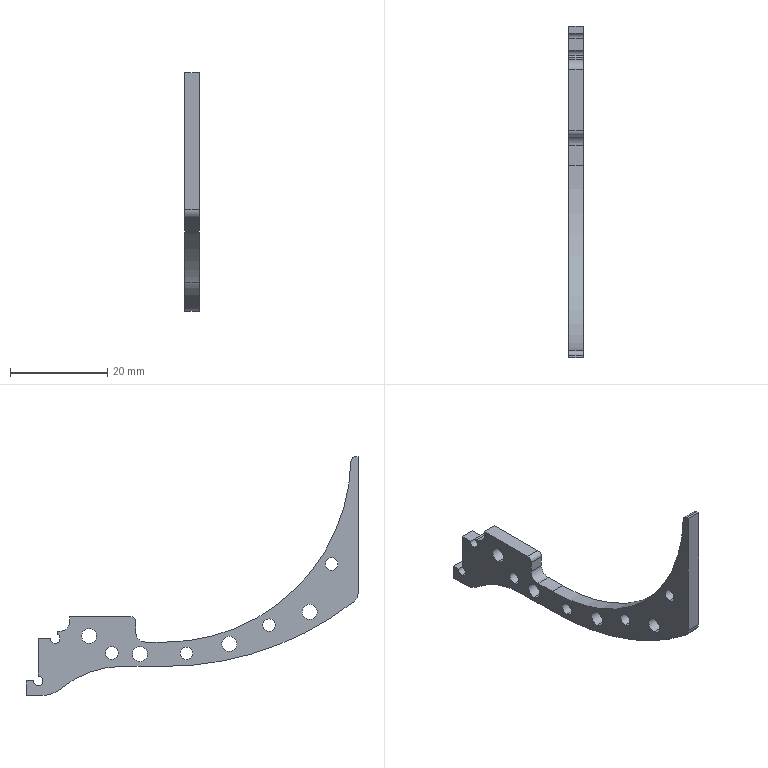Part | SolidWorks | features Fillet 2, Extrusion 1, ICE 1 | 1 solid | 45 faces | box 3 x 68.45 x 49.25 mm | volume 1803 mm3 | cylinder 29 | plane 16 | commonest cylinder face diameters 2.6 x8 3.1 x8 2 x6 4 x3 11.1 x1 40 x1
STEP:
#1=CARTESIAN_POINT('',(0.,27.25,-22.25));
#2=VERTEX_POINT('',#1);
#3=CARTESIAN_POINT('',(0.,26.25,-23.25));
#4=VERTEX_POINT('',#3);
#5=CARTESIAN_POINT('',(0.,26.25,-22.25));
#6=DIRECTION('',(-1.,0.,0.));
#7=DIRECTION('',(0.,0.,-1.));
#8=AXIS2_PLACEMENT_3D('',#5,#6,#7);
#9=CIRCLE('',#8,1.);
#10=EDGE_CURVE('',#2,#4,#9,.T.);
#11=ORIENTED_EDGE('',*,*,#10,.T.);
#12=CARTESIAN_POINT('',(3.,26.25,-23.25));
#13=VERTEX_POINT('',#12);
#14=CARTESIAN_POINT('',(0.,26.25,-23.25));
#15=DIRECTION('',(1.,0.,0.));
#16=VECTOR('',#15,1000.);
#17=LINE('',#14,#16);
#18=EDGE_CURVE('',#4,#13,#17,.T.);
#19=ORIENTED_EDGE('',*,*,#18,.T.);
#20=CARTESIAN_POINT('',(3.,27.25,-22.25));
#21=VERTEX_POINT('',#20);
#22=CARTESIAN_POINT('',(3.,26.25,-22.25));
#23=DIRECTION('',(-1.,0.,0.));
#24=DIRECTION('',(0.,0.,-1.));
#25=AXIS2_PLACEMENT_3D('',#22,#23,#24);
#26=CIRCLE('',#25,1.);
#27=EDGE_CURVE('',#21,#13,#26,.T.);
#28=ORIENTED_EDGE('',*,*,#27,.F.);
#29=CARTESIAN_POINT('',(0.,27.25,-22.25));
#30=DIRECTION('',(1.,0.,0.));
#31=VECTOR('',#30,1000.);
#32=LINE('',#29,#31);
#33=EDGE_CURVE('',#2,#21,#32,.T.);
#34=ORIENTED_EDGE('',*,*,#33,.F.);
#35=EDGE_LOOP('',(#11,#19,#28,#34));
#36=FACE_OUTER_BOUND('',#35,.T.);
#37=CARTESIAN_POINT('',(0.,26.25,-22.25));
#38=DIRECTION('',(1.,0.,0.));
#39=DIRECTION('',(0.,0.,-1.));
#40=AXIS2_PLACEMENT_3D('',#37,#38,#39);
#41=CYLINDRICAL_SURFACE('',#40,1.);
#42=ADVANCED_FACE('',(#36),#41,.F.);
#43=CARTESIAN_POINT('',(0.,23.75,-13.5));
#44=VERTEX_POINT('',#43);
#45=CARTESIAN_POINT('',(0.,22.75,-14.5));
#46=VERTEX_POINT('',#45);
#47=CARTESIAN_POINT('',(0.,22.75,-13.5));
#48=DIRECTION('',(-1.,0.,0.));
#49=DIRECTION('',(0.,0.,-1.));
#50=AXIS2_PLACEMENT_3D('',#47,#48,#49);
#51=CIRCLE('',#50,1.);
#52=EDGE_CURVE('',#44,#46,#51,.T.);
#53=ORIENTED_EDGE('',*,*,#52,.T.);
#54=CARTESIAN_POINT('',(3.,22.75,-14.5));
#55=VERTEX_POINT('',#54);
#56=CARTESIAN_POINT('',(0.,22.75,-14.5));
#57=DIRECTION('',(1.,0.,0.));
#58=VECTOR('',#57,1000.);
#59=LINE('',#56,#58);
#60=EDGE_CURVE('',#46,#55,#59,.T.);
#61=ORIENTED_EDGE('',*,*,#60,.T.);
#62=CARTESIAN_POINT('',(3.,23.75,-13.5));
#63=VERTEX_POINT('',#62);
#64=CARTESIAN_POINT('',(3.,22.75,-13.5));
#65=DIRECTION('',(-1.,0.,0.));
#66=DIRECTION('',(0.,0.,-1.));
#67=AXIS2_PLACEMENT_3D('',#64,#65,#66);
#68=CIRCLE('',#67,1.);
#69=EDGE_CURVE('',#63,#55,#68,.T.);
#70=ORIENTED_EDGE('',*,*,#69,.F.);
#71=CARTESIAN_POINT('',(0.,23.75,-13.5));
#72=DIRECTION('',(1.,0.,0.));
#73=VECTOR('',#72,1000.);
#74=LINE('',#71,#73);
#75=EDGE_CURVE('',#44,#63,#74,.T.);
#76=ORIENTED_EDGE('',*,*,#75,.F.);
#77=EDGE_LOOP('',(#53,#61,#70,#76));
#78=FACE_OUTER_BOUND('',#77,.T.);
#79=CARTESIAN_POINT('',(0.,22.75,-13.5));
#80=DIRECTION('',(1.,0.,0.));
#81=DIRECTION('',(0.,0.,-1.));
#82=AXIS2_PLACEMENT_3D('',#79,#80,#81);
#83=CYLINDRICAL_SURFACE('',#82,1.);
#84=ADVANCED_FACE('',(#78),#83,.F.);
#85=CARTESIAN_POINT('',(3.,15.75,-14.55));
#86=VERTEX_POINT('',#85);
#87=CARTESIAN_POINT('',(3.,15.75,-11.45));
#88=VERTEX_POINT('',#87);
#89=CARTESIAN_POINT('',(3.,15.75,-13.));
#90=DIRECTION('',(-1.,0.,0.));
#91=DIRECTION('',(0.,0.,-1.));
#92=AXIS2_PLACEMENT_3D('',#89,#90,#91);
#93=CIRCLE('',#92,1.55);
#94=EDGE_CURVE('',#86,#88,#93,.T.);
#95=ORIENTED_EDGE('',*,*,#94,.F.);
#96=CARTESIAN_POINT('',(0.,15.75,-14.55));
#97=VERTEX_POINT('',#96);
#98=CARTESIAN_POINT('',(3.,15.75,-14.55));
#99=DIRECTION('',(-1.,0.,0.));
#100=VECTOR('',#99,1000.);
#101=LINE('',#98,#100);
#102=EDGE_CURVE('',#86,#97,#101,.T.);
#103=ORIENTED_EDGE('',*,*,#102,.T.);
#104=CARTESIAN_POINT('',(0.,15.75,-11.45));
#105=VERTEX_POINT('',#104);
#106=CARTESIAN_POINT('',(0.,15.75,-13.));
#107=DIRECTION('',(-1.,0.,0.));
#108=DIRECTION('',(0.,0.,-1.));
#109=AXIS2_PLACEMENT_3D('',#106,#107,#108);
#110=CIRCLE('',#109,1.55);
#111=EDGE_CURVE('',#97,#105,#110,.T.);
#112=ORIENTED_EDGE('',*,*,#111,.T.);
#113=CARTESIAN_POINT('',(3.,15.75,-11.45));
#114=DIRECTION('',(-1.,0.,0.));
#115=VECTOR('',#114,1000.);
#116=LINE('',#113,#115);
#117=EDGE_CURVE('',#88,#105,#116,.T.);
#118=ORIENTED_EDGE('',*,*,#117,.F.);
#119=EDGE_LOOP('',(#95,#103,#112,#118));
#120=FACE_OUTER_BOUND('',#119,.T.);
#121=CARTESIAN_POINT('',(3.,15.75,-13.));
#122=DIRECTION('',(-1.,0.,0.));
#123=DIRECTION('',(0.,0.,1.));
#124=AXIS2_PLACEMENT_3D('',#121,#122,#123);
#125=CYLINDRICAL_SURFACE('',#124,1.55);
#126=ADVANCED_FACE('',(#120),#125,.F.);
#127=CARTESIAN_POINT('',(3.,-29.75,-6.45));
#128=VERTEX_POINT('',#127);
#129=CARTESIAN_POINT('',(3.,-29.75,-9.55));
#130=VERTEX_POINT('',#129);
#131=CARTESIAN_POINT('',(3.,-29.75,-8.));
#132=DIRECTION('',(1.,0.,0.));
#133=DIRECTION('',(0.,0.,-1.));
#134=AXIS2_PLACEMENT_3D('',#131,#132,#133);
#135=CIRCLE('',#134,1.55);
#136=EDGE_CURVE('',#128,#130,#135,.T.);
#137=ORIENTED_EDGE('',*,*,#136,.T.);
#138=CARTESIAN_POINT('',(0.,-29.75,-9.55));
#139=VERTEX_POINT('',#138);
#140=CARTESIAN_POINT('',(3.,-29.75,-9.55));
#141=DIRECTION('',(-1.,0.,0.));
#142=VECTOR('',#141,1000.);
#143=LINE('',#140,#142);
#144=EDGE_CURVE('',#130,#139,#143,.T.);
#145=ORIENTED_EDGE('',*,*,#144,.T.);
#146=CARTESIAN_POINT('',(0.,-29.75,-6.45));
#147=VERTEX_POINT('',#146);
#148=CARTESIAN_POINT('',(0.,-29.75,-8.));
#149=DIRECTION('',(1.,0.,0.));
#150=DIRECTION('',(0.,0.,-1.));
#151=AXIS2_PLACEMENT_3D('',#148,#149,#150);
#152=CIRCLE('',#151,1.55);
#153=EDGE_CURVE('',#147,#139,#152,.T.);
#154=ORIENTED_EDGE('',*,*,#153,.F.);
#155=CARTESIAN_POINT('',(3.,-29.75,-6.45));
#156=DIRECTION('',(-1.,0.,0.));
#157=VECTOR('',#156,1000.);
#158=LINE('',#155,#157);
#159=EDGE_CURVE('',#128,#147,#158,.T.);
#160=ORIENTED_EDGE('',*,*,#159,.F.);
#161=EDGE_LOOP('',(#137,#145,#154,#160));
#162=FACE_OUTER_BOUND('',#161,.T.);
#163=CARTESIAN_POINT('',(3.,-29.75,-8.));
#164=DIRECTION('',(-1.,0.,0.));
#165=DIRECTION('',(0.,0.,1.));
#166=AXIS2_PLACEMENT_3D('',#163,#164,#165);
#167=CYLINDRICAL_SURFACE('',#166,1.55);
#168=ADVANCED_FACE('',(#162),#167,.F.);
#169=CARTESIAN_POINT('',(3.,-4.324,-15.27));
#170=VERTEX_POINT('',#169);
#171=CARTESIAN_POINT('',(3.,-4.324,-17.87));
#172=VERTEX_POINT('',#171);
#173=CARTESIAN_POINT('',(3.,-4.324,-16.57));
#174=DIRECTION('',(1.,0.,0.));
#175=DIRECTION('',(0.,0.,-1.));
#176=AXIS2_PLACEMENT_3D('',#173,#174,#175);
#177=CIRCLE('',#176,1.3);
#178=EDGE_CURVE('',#170,#172,#177,.T.);
#179=ORIENTED_EDGE('',*,*,#178,.T.);
#180=CARTESIAN_POINT('',(0.,-4.324,-17.87));
#181=VERTEX_POINT('',#180);
#182=CARTESIAN_POINT('',(3.,-4.324,-17.87));
#183=DIRECTION('',(-1.,0.,0.));
#184=VECTOR('',#183,1000.);
#185=LINE('',#182,#184);
#186=EDGE_CURVE('',#172,#181,#185,.T.);
#187=ORIENTED_EDGE('',*,*,#186,.T.);
#188=CARTESIAN_POINT('',(0.,-4.324,-15.27));
#189=VERTEX_POINT('',#188);
#190=CARTESIAN_POINT('',(0.,-4.324,-16.57));
#191=DIRECTION('',(1.,0.,0.));
#192=DIRECTION('',(0.,0.,-1.));
#193=AXIS2_PLACEMENT_3D('',#190,#191,#192);
#194=CIRCLE('',#193,1.3);
#195=EDGE_CURVE('',#189,#181,#194,.T.);
#196=ORIENTED_EDGE('',*,*,#195,.F.);
#197=CARTESIAN_POINT('',(3.,-4.324,-15.27));
#198=DIRECTION('',(-1.,0.,0.));
#199=VECTOR('',#198,1000.);
#200=LINE('',#197,#199);
#201=EDGE_CURVE('',#170,#189,#200,.T.);
#202=ORIENTED_EDGE('',*,*,#201,.F.);
#203=EDGE_LOOP('',(#179,#187,#196,#202));
#204=FACE_OUTER_BOUND('',#203,.T.);
#205=CARTESIAN_POINT('',(3.,-4.324,-16.57));
#206=DIRECTION('',(-1.,0.,0.));
#207=DIRECTION('',(0.,0.,1.));
#208=AXIS2_PLACEMENT_3D('',#205,#206,#207);
#209=CYLINDRICAL_SURFACE('',#208,1.3);
#210=ADVANCED_FACE('',(#204),#209,.F.);
#211=CARTESIAN_POINT('',(3.,-13.171,-13.066));
#212=VERTEX_POINT('',#211);
#213=CARTESIAN_POINT('',(3.,-13.171,-16.166));
#214=VERTEX_POINT('',#213);
#215=CARTESIAN_POINT('',(3.,-13.171,-14.616));
#216=DIRECTION('',(1.,0.,0.));
#217=DIRECTION('',(0.,0.,-1.));
#218=AXIS2_PLACEMENT_3D('',#215,#216,#217);
#219=CIRCLE('',#218,1.55);
#220=EDGE_CURVE('',#212,#214,#219,.T.);
#221=ORIENTED_EDGE('',*,*,#220,.T.);
#222=CARTESIAN_POINT('',(0.,-13.171,-16.166));
#223=VERTEX_POINT('',#222);
#224=CARTESIAN_POINT('',(3.,-13.171,-16.166));
#225=DIRECTION('',(-1.,0.,0.));
#226=VECTOR('',#225,1000.);
#227=LINE('',#224,#226);
#228=EDGE_CURVE('',#214,#223,#227,.T.);
#229=ORIENTED_EDGE('',*,*,#228,.T.);
#230=CARTESIAN_POINT('',(0.,-13.171,-13.066));
#231=VERTEX_POINT('',#230);
#232=CARTESIAN_POINT('',(0.,-13.171,-14.616));
#233=DIRECTION('',(1.,0.,0.));
#234=DIRECTION('',(0.,0.,-1.));
#235=AXIS2_PLACEMENT_3D('',#232,#233,#234);
#236=CIRCLE('',#235,1.55);
#237=EDGE_CURVE('',#231,#223,#236,.T.);
#238=ORIENTED_EDGE('',*,*,#237,.F.);
#239=CARTESIAN_POINT('',(3.,-13.171,-13.066));
#240=DIRECTION('',(-1.,0.,0.));
#241=VECTOR('',#240,1000.);
#242=LINE('',#239,#241);
#243=EDGE_CURVE('',#212,#231,#242,.T.);
#244=ORIENTED_EDGE('',*,*,#243,.F.);
#245=EDGE_LOOP('',(#221,#229,#238,#244));
#246=FACE_OUTER_BOUND('',#245,.T.);
#247=CARTESIAN_POINT('',(3.,-13.171,-14.616));
#248=DIRECTION('',(-1.,0.,0.));
#249=DIRECTION('',(0.,0.,1.));
#250=AXIS2_PLACEMENT_3D('',#247,#248,#249);
#251=CYLINDRICAL_SURFACE('',#250,1.55);
#252=ADVANCED_FACE('',(#246),#251,.F.);
#253=CARTESIAN_POINT('',(3.,-21.368,-9.457));
#254=VERTEX_POINT('',#253);
#255=CARTESIAN_POINT('',(3.,-21.368,-12.057));
#256=VERTEX_POINT('',#255);
#257=CARTESIAN_POINT('',(3.,-21.368,-10.757));
#258=DIRECTION('',(1.,0.,0.));
#259=DIRECTION('',(0.,0.,-1.));
#260=AXIS2_PLACEMENT_3D('',#257,#258,#259);
#261=CIRCLE('',#260,1.3);
#262=EDGE_CURVE('',#254,#256,#261,.T.);
#263=ORIENTED_EDGE('',*,*,#262,.T.);
#264=CARTESIAN_POINT('',(0.,-21.368,-12.057));
#265=VERTEX_POINT('',#264);
#266=CARTESIAN_POINT('',(3.,-21.368,-12.057));
#267=DIRECTION('',(-1.,0.,0.));
#268=VECTOR('',#267,1000.);
#269=LINE('',#266,#268);
#270=EDGE_CURVE('',#256,#265,#269,.T.);
#271=ORIENTED_EDGE('',*,*,#270,.T.);
#272=CARTESIAN_POINT('',(0.,-21.368,-9.457));
#273=VERTEX_POINT('',#272);
#274=CARTESIAN_POINT('',(0.,-21.368,-10.757));
#275=DIRECTION('',(1.,0.,0.));
#276=DIRECTION('',(0.,0.,-1.));
#277=AXIS2_PLACEMENT_3D('',#274,#275,#276);
#278=CIRCLE('',#277,1.3);
#279=EDGE_CURVE('',#273,#265,#278,.T.);
#280=ORIENTED_EDGE('',*,*,#279,.F.);
#281=CARTESIAN_POINT('',(3.,-21.368,-9.457));
#282=DIRECTION('',(-1.,0.,0.));
#283=VECTOR('',#282,1000.);
#284=LINE('',#281,#283);
#285=EDGE_CURVE('',#254,#273,#284,.T.);
#286=ORIENTED_EDGE('',*,*,#285,.F.);
#287=EDGE_LOOP('',(#263,#271,#280,#286));
#288=FACE_OUTER_BOUND('',#287,.T.);
#289=CARTESIAN_POINT('',(3.,-21.368,-10.757));
#290=DIRECTION('',(-1.,0.,0.));
#291=DIRECTION('',(0.,0.,1.));
#292=AXIS2_PLACEMENT_3D('',#289,#290,#291);
#293=CYLINDRICAL_SURFACE('',#292,1.3);
#294=ADVANCED_FACE('',(#288),#293,.F.);
#295=CARTESIAN_POINT('',(3.,-34.25,3.128));
#296=VERTEX_POINT('',#295);
#297=CARTESIAN_POINT('',(3.,-34.25,0.5285));
#298=VERTEX_POINT('',#297);
#299=CARTESIAN_POINT('',(3.,-34.25,1.828));
#300=DIRECTION('',(1.,0.,0.));
#301=DIRECTION('',(0.,0.,-1.));
#302=AXIS2_PLACEMENT_3D('',#299,#300,#301);
#303=CIRCLE('',#302,1.3);
#304=EDGE_CURVE('',#296,#298,#303,.T.);
#305=ORIENTED_EDGE('',*,*,#304,.T.);
#306=CARTESIAN_POINT('',(0.,-34.25,0.5285));
#307=VERTEX_POINT('',#306);
#308=CARTESIAN_POINT('',(3.,-34.25,0.5285));
#309=DIRECTION('',(-1.,0.,0.));
#310=VECTOR('',#309,1000.);
#311=LINE('',#308,#310);
#312=EDGE_CURVE('',#298,#307,#311,.T.);
#313=ORIENTED_EDGE('',*,*,#312,.T.);
#314=CARTESIAN_POINT('',(0.,-34.25,3.128));
#315=VERTEX_POINT('',#314);
#316=CARTESIAN_POINT('',(0.,-34.25,1.828));
#317=DIRECTION('',(1.,0.,0.));
#318=DIRECTION('',(0.,0.,-1.));
#319=AXIS2_PLACEMENT_3D('',#316,#317,#318);
#320=CIRCLE('',#319,1.3);
#321=EDGE_CURVE('',#315,#307,#320,.T.);
#322=ORIENTED_EDGE('',*,*,#321,.F.);
#323=CARTESIAN_POINT('',(3.,-34.25,3.128));
#324=DIRECTION('',(-1.,0.,0.));
#325=VECTOR('',#324,1000.);
#326=LINE('',#323,#325);
#327=EDGE_CURVE('',#296,#315,#326,.T.);
#328=ORIENTED_EDGE('',*,*,#327,.F.);
#329=EDGE_LOOP('',(#305,#313,#322,#328));
#330=FACE_OUTER_BOUND('',#329,.T.);
#331=CARTESIAN_POINT('',(3.,-34.25,1.828));
#332=DIRECTION('',(-1.,0.,0.));
#333=DIRECTION('',(0.,0.,1.));
#334=AXIS2_PLACEMENT_3D('',#331,#332,#333);
#335=CYLINDRICAL_SURFACE('',#334,1.3);
#336=ADVANCED_FACE('',(#330),#335,.F.);
#337=CARTESIAN_POINT('',(3.,5.25,-15.2));
#338=VERTEX_POINT('',#337);
#339=CARTESIAN_POINT('',(3.,5.25,-18.3));
#340=VERTEX_POINT('',#339);
#341=CARTESIAN_POINT('',(3.,5.25,-16.75));
#342=DIRECTION('',(1.,0.,0.));
#343=DIRECTION('',(0.,0.,-1.));
#344=AXIS2_PLACEMENT_3D('',#341,#342,#343);
#345=CIRCLE('',#344,1.55);
#346=EDGE_CURVE('',#338,#340,#345,.T.);
#347=ORIENTED_EDGE('',*,*,#346,.T.);
#348=CARTESIAN_POINT('',(0.,5.25,-18.3));
#349=VERTEX_POINT('',#348);
#350=CARTESIAN_POINT('',(3.,5.25,-18.3));
#351=DIRECTION('',(-1.,0.,0.));
#352=VECTOR('',#351,1000.);
#353=LINE('',#350,#352);
#354=EDGE_CURVE('',#340,#349,#353,.T.);
#355=ORIENTED_EDGE('',*,*,#354,.T.);
#356=CARTESIAN_POINT('',(0.,5.25,-15.2));
#357=VERTEX_POINT('',#356);
#358=CARTESIAN_POINT('',(0.,5.25,-16.75));
#359=DIRECTION('',(1.,0.,0.));
#360=DIRECTION('',(0.,0.,-1.));
#361=AXIS2_PLACEMENT_3D('',#358,#359,#360);
#362=CIRCLE('',#361,1.55);
#363=EDGE_CURVE('',#357,#349,#362,.T.);
#364=ORIENTED_EDGE('',*,*,#363,.F.);
#365=CARTESIAN_POINT('',(3.,5.25,-15.2));
#366=DIRECTION('',(-1.,0.,0.));
#367=VECTOR('',#366,1000.);
#368=LINE('',#365,#367);
#369=EDGE_CURVE('',#338,#357,#368,.T.);
#370=ORIENTED_EDGE('',*,*,#369,.F.);
#371=EDGE_LOOP('',(#347,#355,#364,#370));
#372=FACE_OUTER_BOUND('',#371,.T.);
#373=CARTESIAN_POINT('',(3.,5.25,-16.75));
#374=DIRECTION('',(-1.,0.,0.));
#375=DIRECTION('',(0.,0.,1.));
#376=AXIS2_PLACEMENT_3D('',#373,#374,#375);
#377=CYLINDRICAL_SURFACE('',#376,1.55);
#378=ADVANCED_FACE('',(#372),#377,.F.);
#379=CARTESIAN_POINT('',(3.,11.05,-17.8));
#380=VERTEX_POINT('',#379);
#381=CARTESIAN_POINT('',(3.,11.05,-15.2));
#382=VERTEX_POINT('',#381);
#383=CARTESIAN_POINT('',(3.,11.05,-16.5));
#384=DIRECTION('',(-1.,0.,0.));
#385=DIRECTION('',(0.,0.,-1.));
#386=AXIS2_PLACEMENT_3D('',#383,#384,#385);
#387=CIRCLE('',#386,1.3);
#388=EDGE_CURVE('',#380,#382,#387,.T.);
#389=ORIENTED_EDGE('',*,*,#388,.F.);
#390=CARTESIAN_POINT('',(0.,11.05,-17.8));
#391=VERTEX_POINT('',#390);
#392=CARTESIAN_POINT('',(3.,11.05,-17.8));
#393=DIRECTION('',(-1.,0.,0.));
#394=VECTOR('',#393,1000.);
#395=LINE('',#392,#394);
#396=EDGE_CURVE('',#380,#391,#395,.T.);
#397=ORIENTED_EDGE('',*,*,#396,.T.);
#398=CARTESIAN_POINT('',(0.,11.05,-15.2));
#399=VERTEX_POINT('',#398);
#400=CARTESIAN_POINT('',(0.,11.05,-16.5));
#401=DIRECTION('',(-1.,0.,0.));
#402=DIRECTION('',(0.,0.,-1.));
#403=AXIS2_PLACEMENT_3D('',#400,#401,#402);
#404=CIRCLE('',#403,1.3);
#405=EDGE_CURVE('',#391,#399,#404,.T.);
#406=ORIENTED_EDGE('',*,*,#405,.T.);
#407=CARTESIAN_POINT('',(3.,11.05,-15.2));
#408=DIRECTION('',(-1.,0.,0.));
#409=VECTOR('',#408,1000.);
#410=LINE('',#407,#409);
#411=EDGE_CURVE('',#382,#399,#410,.T.);
#412=ORIENTED_EDGE('',*,*,#411,.F.);
#413=EDGE_LOOP('',(#389,#397,#406,#412));
#414=FACE_OUTER_BOUND('',#413,.T.);
#415=CARTESIAN_POINT('',(3.,11.05,-16.5));
#416=DIRECTION('',(-1.,0.,0.));
#417=DIRECTION('',(0.,0.,1.));
#418=AXIS2_PLACEMENT_3D('',#415,#416,#417);
#419=CYLINDRICAL_SURFACE('',#418,1.3);
#420=ADVANCED_FACE('',(#414),#419,.F.);
#421=CARTESIAN_POINT('',(3.,19.75,-9.));
#422=VERTEX_POINT('',#421);
#423=CARTESIAN_POINT('',(3.,19.75,-10.));
#424=VERTEX_POINT('',#423);
#425=CARTESIAN_POINT('',(3.,19.75,0.));
#426=DIRECTION('',(0.,0.,-1.));
#427=VECTOR('',#426,1000.);
#428=LINE('',#425,#427);
#429=EDGE_CURVE('',#422,#424,#428,.T.);
#430=ORIENTED_EDGE('',*,*,#429,.T.);
#431=CARTESIAN_POINT('',(0.,19.75,-10.));
#432=VERTEX_POINT('',#431);
#433=CARTESIAN_POINT('',(0.,19.75,-10.));
#434=DIRECTION('',(-1.,0.,0.));
#435=VECTOR('',#434,1000.);
#436=LINE('',#433,#435);
#437=EDGE_CURVE('',#424,#432,#436,.T.);
#438=ORIENTED_EDGE('',*,*,#437,.T.);
#439=CARTESIAN_POINT('',(0.,19.75,-9.));
#440=VERTEX_POINT('',#439);
#441=CARTESIAN_POINT('',(0.,19.75,0.));
#442=DIRECTION('',(0.,0.,-1.));
#443=VECTOR('',#442,1000.);
#444=LINE('',#441,#443);
#445=EDGE_CURVE('',#440,#432,#444,.T.);
#446=ORIENTED_EDGE('',*,*,#445,.F.);
#447=CARTESIAN_POINT('',(0.,19.75,-9.));
#448=DIRECTION('',(1.,0.,0.));
#449=VECTOR('',#448,1000.);
#450=LINE('',#447,#449);
#451=EDGE_CURVE('',#440,#422,#450,.T.);
#452=ORIENTED_EDGE('',*,*,#451,.T.);
#453=EDGE_LOOP('',(#430,#438,#446,#452));
#454=FACE_OUTER_BOUND('',#453,.T.);
#455=CARTESIAN_POINT('',(3.,19.75,0.));
#456=DIRECTION('',(0.,1.,0.));
#457=DIRECTION('',(0.,0.,1.));
#458=AXIS2_PLACEMENT_3D('',#455,#456,#457);
#459=PLANE('',#458);
#460=ADVANCED_FACE('',(#454),#459,.T.);
#461=CARTESIAN_POINT('',(3.,6.116,-10.));
#462=VERTEX_POINT('',#461);
#463=CARTESIAN_POINT('',(3.,6.116,-12.25));
#464=VERTEX_POINT('',#463);
#465=CARTESIAN_POINT('',(3.,6.116,0.));
#466=DIRECTION('',(0.,0.,-1.));
#467=VECTOR('',#466,1000.);
#468=LINE('',#465,#467);
#469=EDGE_CURVE('',#462,#464,#468,.T.);
#470=ORIENTED_EDGE('',*,*,#469,.F.);
#471=CARTESIAN_POINT('',(0.,6.116,-10.));
#472=VERTEX_POINT('',#471);
#473=CARTESIAN_POINT('',(0.,6.116,-10.));
#474=DIRECTION('',(-1.,0.,0.));
#475=VECTOR('',#474,1000.);
#476=LINE('',#473,#475);
#477=EDGE_CURVE('',#462,#472,#476,.T.);
#478=ORIENTED_EDGE('',*,*,#477,.T.);
#479=CARTESIAN_POINT('',(0.,6.116,-12.25));
#480=VERTEX_POINT('',#479);
#481=CARTESIAN_POINT('',(0.,6.116,0.));
#482=DIRECTION('',(0.,0.,-1.));
#483=VECTOR('',#482,1000.);
#484=LINE('',#481,#483);
#485=EDGE_CURVE('',#472,#480,#484,.T.);
#486=ORIENTED_EDGE('',*,*,#485,.T.);
#487=CARTESIAN_POINT('',(3.,6.116,-12.25));
#488=DIRECTION('',(1.,0.,0.));
#489=VECTOR('',#488,1000.);
#490=LINE('',#487,#489);
#491=EDGE_CURVE('',#480,#464,#490,.T.);
#492=ORIENTED_EDGE('',*,*,#491,.T.);
#493=EDGE_LOOP('',(#470,#478,#486,#492));
#494=FACE_OUTER_BOUND('',#493,.T.);
#495=CARTESIAN_POINT('',(3.,6.116,0.));
#496=DIRECTION('',(0.,1.,0.));
#497=DIRECTION('',(0.,0.,1.));
#498=AXIS2_PLACEMENT_3D('',#495,#496,#497);
#499=PLANE('',#498);
#500=ADVANCED_FACE('',(#494),#499,.F.);
#501=CARTESIAN_POINT('',(3.,0.,-14.25));
#502=VERTEX_POINT('',#501);
#503=CARTESIAN_POINT('',(3.,4.116,-14.25));
#504=VERTEX_POINT('',#503);
#505=CARTESIAN_POINT('',(3.,0.,-14.25));
#506=DIRECTION('',(0.,1.,0.));
#507=VECTOR('',#506,1000.);
#508=LINE('',#505,#507);
#509=EDGE_CURVE('',#502,#504,#508,.T.);
#510=ORIENTED_EDGE('',*,*,#509,.T.);
#511=CARTESIAN_POINT('',(0.,4.116,-14.25));
#512=VERTEX_POINT('',#511);
#513=CARTESIAN_POINT('',(3.,4.116,-14.25));
#514=DIRECTION('',(-1.,0.,0.));
#515=VECTOR('',#514,1000.);
#516=LINE('',#513,#515);
#517=EDGE_CURVE('',#504,#512,#516,.T.);
#518=ORIENTED_EDGE('',*,*,#517,.T.);
#519=CARTESIAN_POINT('',(0.,0.,-14.25));
#520=VERTEX_POINT('',#519);
#521=CARTESIAN_POINT('',(0.,0.,-14.25));
#522=DIRECTION('',(0.,1.,0.));
#523=VECTOR('',#522,1000.);
#524=LINE('',#521,#523);
#525=EDGE_CURVE('',#520,#512,#524,.T.);
#526=ORIENTED_EDGE('',*,*,#525,.F.);
#527=CARTESIAN_POINT('',(3.,0.,-14.25));
#528=DIRECTION('',(-1.,0.,0.));
#529=VECTOR('',#528,1000.);
#530=LINE('',#527,#529);
#531=EDGE_CURVE('',#502,#520,#530,.T.);
#532=ORIENTED_EDGE('',*,*,#531,.F.);
#533=EDGE_LOOP('',(#510,#518,#526,#532));
#534=FACE_OUTER_BOUND('',#533,.T.);
#535=CARTESIAN_POINT('',(3.,0.,-14.25));
#536=DIRECTION('',(0.,0.,1.));
#537=DIRECTION('',(0.,-1.,0.));
#538=AXIS2_PLACEMENT_3D('',#535,#536,#537);
#539=PLANE('',#538);
#540=ADVANCED_FACE('',(#534),#539,.T.);
#541=CARTESIAN_POINT('',(0.,-38.238,23.025));
#542=VERTEX_POINT('',#541);
#543=CARTESIAN_POINT('',(0.,0.,24.));
#544=DIRECTION('',(1.,0.,0.));
#545=DIRECTION('',(0.,0.,-1.));
#546=AXIS2_PLACEMENT_3D('',#543,#544,#545);
#547=CIRCLE('',#546,38.25);
#548=EDGE_CURVE('',#542,#520,#547,.T.);
#549=ORIENTED_EDGE('',*,*,#548,.F.);
#550=CARTESIAN_POINT('',(3.,-38.238,23.025));
#551=VERTEX_POINT('',#550);
#552=CARTESIAN_POINT('',(3.,-38.238,23.025));
#553=DIRECTION('',(1.,0.,0.));
#554=VECTOR('',#553,1000.);
#555=LINE('',#552,#554);
#556=EDGE_CURVE('',#542,#551,#555,.T.);
#557=ORIENTED_EDGE('',*,*,#556,.T.);
#558=CARTESIAN_POINT('',(3.,0.,24.));
#559=DIRECTION('',(1.,0.,0.));
#560=DIRECTION('',(0.,0.,-1.));
#561=AXIS2_PLACEMENT_3D('',#558,#559,#560);
#562=CIRCLE('',#561,38.25);
#563=EDGE_CURVE('',#551,#502,#562,.T.);
#564=ORIENTED_EDGE('',*,*,#563,.T.);
#565=ORIENTED_EDGE('',*,*,#531,.T.);
#566=EDGE_LOOP('',(#549,#557,#564,#565));
#567=FACE_OUTER_BOUND('',#566,.T.);
#568=CARTESIAN_POINT('',(3.,0.,24.));
#569=DIRECTION('',(-1.,0.,0.));
#570=DIRECTION('',(0.,0.,1.));
#571=AXIS2_PLACEMENT_3D('',#568,#569,#570);
#572=CYLINDRICAL_SURFACE('',#571,38.25);
#573=ADVANCED_FACE('',(#567),#572,.F.);
#574=CARTESIAN_POINT('',(3.,-39.7,24.));
#575=VERTEX_POINT('',#574);
#576=CARTESIAN_POINT('',(3.,-39.237,24.));
#577=VERTEX_POINT('',#576);
#578=CARTESIAN_POINT('',(3.,0.,24.));
#579=DIRECTION('',(0.,1.,0.));
#580=VECTOR('',#579,1000.);
#581=LINE('',#578,#580);
#582=EDGE_CURVE('',#575,#577,#581,.T.);
#583=ORIENTED_EDGE('',*,*,#582,.T.);
#584=CARTESIAN_POINT('',(0.,-39.237,24.));
#585=VERTEX_POINT('',#584);
#586=CARTESIAN_POINT('',(3.,-39.237,24.));
#587=DIRECTION('',(-1.,0.,0.));
#588=VECTOR('',#587,1000.);
#589=LINE('',#586,#588);
#590=EDGE_CURVE('',#577,#585,#589,.T.);
#591=ORIENTED_EDGE('',*,*,#590,.T.);
#592=CARTESIAN_POINT('',(0.,-39.7,24.));
#593=VERTEX_POINT('',#592);
#594=CARTESIAN_POINT('',(0.,0.,24.));
#595=DIRECTION('',(0.,1.,0.));
#596=VECTOR('',#595,1000.);
#597=LINE('',#594,#596);
#598=EDGE_CURVE('',#593,#585,#597,.T.);
#599=ORIENTED_EDGE('',*,*,#598,.F.);
#600=CARTESIAN_POINT('',(3.,-39.7,24.));
#601=DIRECTION('',(-1.,0.,0.));
#602=VECTOR('',#601,1000.);
#603=LINE('',#600,#602);
#604=EDGE_CURVE('',#575,#593,#603,.T.);
#605=ORIENTED_EDGE('',*,*,#604,.F.);
#606=EDGE_LOOP('',(#583,#591,#599,#605));
#607=FACE_OUTER_BOUND('',#606,.T.);
#608=CARTESIAN_POINT('',(3.,0.,24.));
#609=DIRECTION('',(0.,0.,1.));
#610=DIRECTION('',(0.,-1.,0.));
#611=AXIS2_PLACEMENT_3D('',#608,#609,#610);
#612=PLANE('',#611);
#613=ADVANCED_FACE('',(#607),#612,.T.);
#614=CARTESIAN_POINT('',(0.,-39.7,-4.273));
#615=VERTEX_POINT('',#614);
#616=CARTESIAN_POINT('',(0.,-39.7,0.));
#617=DIRECTION('',(0.,0.,1.));
#618=VECTOR('',#617,1000.);
#619=LINE('',#616,#618);
#620=EDGE_CURVE('',#615,#593,#619,.T.);
#621=ORIENTED_EDGE('',*,*,#620,.F.);
#622=CARTESIAN_POINT('',(3.,-39.7,-4.273));
#623=VERTEX_POINT('',#622);
#624=CARTESIAN_POINT('',(3.,-39.7,-4.273));
#625=DIRECTION('',(1.,0.,0.));
#626=VECTOR('',#625,1000.);
#627=LINE('',#624,#626);
#628=EDGE_CURVE('',#615,#623,#627,.T.);
#629=ORIENTED_EDGE('',*,*,#628,.T.);
#630=CARTESIAN_POINT('',(3.,-39.7,0.));
#631=DIRECTION('',(0.,0.,1.));
#632=VECTOR('',#631,1000.);
#633=LINE('',#630,#632);
#634=EDGE_CURVE('',#623,#575,#633,.T.);
#635=ORIENTED_EDGE('',*,*,#634,.T.);
#636=ORIENTED_EDGE('',*,*,#604,.T.);
#637=EDGE_LOOP('',(#621,#629,#635,#636));
#638=FACE_OUTER_BOUND('',#637,.T.);
#639=CARTESIAN_POINT('',(3.,-39.7,0.));
#640=DIRECTION('',(0.,-1.,0.));
#641=DIRECTION('',(0.,0.,-1.));
#642=AXIS2_PLACEMENT_3D('',#639,#640,#641);
#643=PLANE('',#642);
#644=ADVANCED_FACE('',(#638),#643,.T.);
#645=CARTESIAN_POINT('',(3.,-38.931,-5.849));
#646=VERTEX_POINT('',#645);
#647=CARTESIAN_POINT('',(3.,0.,-19.25));
#648=VERTEX_POINT('',#647);
#649=CARTESIAN_POINT('',(3.,0.,44.));
#650=DIRECTION('',(1.,0.,0.));
#651=DIRECTION('',(0.,0.,-1.));
#652=AXIS2_PLACEMENT_3D('',#649,#650,#651);
#653=CIRCLE('',#652,63.25);
#654=EDGE_CURVE('',#646,#648,#653,.T.);
#655=ORIENTED_EDGE('',*,*,#654,.F.);
#656=CARTESIAN_POINT('',(0.,-38.931,-5.849));
#657=VERTEX_POINT('',#656);
#658=CARTESIAN_POINT('',(3.,-38.931,-5.849));
#659=DIRECTION('',(-1.,0.,0.));
#660=VECTOR('',#659,1000.);
#661=LINE('',#658,#660);
#662=EDGE_CURVE('',#646,#657,#661,.T.);
#663=ORIENTED_EDGE('',*,*,#662,.T.);
#664=CARTESIAN_POINT('',(0.,0.,-19.25));
#665=VERTEX_POINT('',#664);
#666=CARTESIAN_POINT('',(0.,0.,44.));
#667=DIRECTION('',(1.,0.,0.));
#668=DIRECTION('',(0.,0.,-1.));
#669=AXIS2_PLACEMENT_3D('',#666,#667,#668);
#670=CIRCLE('',#669,63.25);
#671=EDGE_CURVE('',#657,#665,#670,.T.);
#672=ORIENTED_EDGE('',*,*,#671,.T.);
#673=CARTESIAN_POINT('',(3.,0.,-19.25));
#674=DIRECTION('',(-1.,0.,0.));
#675=VECTOR('',#674,1000.);
#676=LINE('',#673,#675);
#677=EDGE_CURVE('',#648,#665,#676,.T.);
#678=ORIENTED_EDGE('',*,*,#677,.F.);
#679=EDGE_LOOP('',(#655,#663,#672,#678));
#680=FACE_OUTER_BOUND('',#679,.T.);
#681=CARTESIAN_POINT('',(3.,0.,44.));
#682=DIRECTION('',(-1.,0.,0.));
#683=DIRECTION('',(0.,0.,1.));
#684=AXIS2_PLACEMENT_3D('',#681,#682,#683);
#685=CYLINDRICAL_SURFACE('',#684,63.25);
#686=ADVANCED_FACE('',(#680),#685,.T.);
#687=ORIENTED_EDGE('',*,*,#396,.F.);
#688=CARTESIAN_POINT('',(3.,11.05,-16.5));
#689=DIRECTION('',(-1.,0.,0.));
#690=DIRECTION('',(0.,0.,-1.));
#691=AXIS2_PLACEMENT_3D('',#688,#689,#690);
#692=CIRCLE('',#691,1.3);
#693=EDGE_CURVE('',#382,#380,#692,.T.);
#694=ORIENTED_EDGE('',*,*,#693,.F.);
#695=ORIENTED_EDGE('',*,*,#411,.T.);
#696=CARTESIAN_POINT('',(0.,11.05,-16.5));
#697=DIRECTION('',(-1.,0.,0.));
#698=DIRECTION('',(0.,0.,-1.));
#699=AXIS2_PLACEMENT_3D('',#696,#697,#698);
#700=CIRCLE('',#699,1.3);
#701=EDGE_CURVE('',#399,#391,#700,.T.);
#702=ORIENTED_EDGE('',*,*,#701,.T.);
#703=EDGE_LOOP('',(#687,#694,#695,#702));
#704=FACE_OUTER_BOUND('',#703,.T.);
#705=CARTESIAN_POINT('',(3.,11.05,-16.5));
#706=DIRECTION('',(-1.,0.,0.));
#707=DIRECTION('',(0.,0.,1.));
#708=AXIS2_PLACEMENT_3D('',#705,#706,#707);
#709=CYLINDRICAL_SURFACE('',#708,1.3);
#710=ADVANCED_FACE('',(#704),#709,.F.);
#711=ORIENTED_EDGE('',*,*,#354,.F.);
#712=CARTESIAN_POINT('',(3.,5.25,-16.75));
#713=DIRECTION('',(1.,0.,0.));
#714=DIRECTION('',(0.,0.,-1.));
#715=AXIS2_PLACEMENT_3D('',#712,#713,#714);
#716=CIRCLE('',#715,1.55);
#717=EDGE_CURVE('',#340,#338,#716,.T.);
#718=ORIENTED_EDGE('',*,*,#717,.T.);
#719=ORIENTED_EDGE('',*,*,#369,.T.);
#720=CARTESIAN_POINT('',(0.,5.25,-16.75));
#721=DIRECTION('',(1.,0.,0.));
#722=DIRECTION('',(0.,0.,-1.));
#723=AXIS2_PLACEMENT_3D('',#720,#721,#722);
#724=CIRCLE('',#723,1.55);
#725=EDGE_CURVE('',#349,#357,#724,.T.);
#726=ORIENTED_EDGE('',*,*,#725,.F.);
#727=EDGE_LOOP('',(#711,#718,#719,#726));
#728=FACE_OUTER_BOUND('',#727,.T.);
#729=CARTESIAN_POINT('',(3.,5.25,-16.75));
#730=DIRECTION('',(-1.,0.,0.));
#731=DIRECTION('',(0.,0.,1.));
#732=AXIS2_PLACEMENT_3D('',#729,#730,#731);
#733=CYLINDRICAL_SURFACE('',#732,1.55);
#734=ADVANCED_FACE('',(#728),#733,.F.);
#735=ORIENTED_EDGE('',*,*,#312,.F.);
#736=CARTESIAN_POINT('',(3.,-34.25,1.828));
#737=DIRECTION('',(1.,0.,0.));
#738=DIRECTION('',(0.,0.,-1.));
#739=AXIS2_PLACEMENT_3D('',#736,#737,#738);
#740=CIRCLE('',#739,1.3);
#741=EDGE_CURVE('',#298,#296,#740,.T.);
#742=ORIENTED_EDGE('',*,*,#741,.T.);
#743=ORIENTED_EDGE('',*,*,#327,.T.);
#744=CARTESIAN_POINT('',(0.,-34.25,1.828));
#745=DIRECTION('',(1.,0.,0.));
#746=DIRECTION('',(0.,0.,-1.));
#747=AXIS2_PLACEMENT_3D('',#744,#745,#746);
#748=CIRCLE('',#747,1.3);
#749=EDGE_CURVE('',#307,#315,#748,.T.);
#750=ORIENTED_EDGE('',*,*,#749,.F.);
#751=EDGE_LOOP('',(#735,#742,#743,#750));
#752=FACE_OUTER_BOUND('',#751,.T.);
#753=CARTESIAN_POINT('',(3.,-34.25,1.828));
#754=DIRECTION('',(-1.,0.,0.));
#755=DIRECTION('',(0.,0.,1.));
#756=AXIS2_PLACEMENT_3D('',#753,#754,#755);
#757=CYLINDRICAL_SURFACE('',#756,1.3);
#758=ADVANCED_FACE('',(#752),#757,.F.);
#759=ORIENTED_EDGE('',*,*,#270,.F.);
#760=CARTESIAN_POINT('',(3.,-21.368,-10.757));
#761=DIRECTION('',(1.,0.,0.));
#762=DIRECTION('',(0.,0.,-1.));
#763=AXIS2_PLACEMENT_3D('',#760,#761,#762);
#764=CIRCLE('',#763,1.3);
#765=EDGE_CURVE('',#256,#254,#764,.T.);
#766=ORIENTED_EDGE('',*,*,#765,.T.);
#767=ORIENTED_EDGE('',*,*,#285,.T.);
#768=CARTESIAN_POINT('',(0.,-21.368,-10.757));
#769=DIRECTION('',(1.,0.,0.));
#770=DIRECTION('',(0.,0.,-1.));
#771=AXIS2_PLACEMENT_3D('',#768,#769,#770);
#772=CIRCLE('',#771,1.3);
#773=EDGE_CURVE('',#265,#273,#772,.T.);
#774=ORIENTED_EDGE('',*,*,#773,.F.);
#775=EDGE_LOOP('',(#759,#766,#767,#774));
#776=FACE_OUTER_BOUND('',#775,.T.);
#777=CARTESIAN_POINT('',(3.,-21.368,-10.757));
#778=DIRECTION('',(-1.,0.,0.));
#779=DIRECTION('',(0.,0.,1.));
#780=AXIS2_PLACEMENT_3D('',#777,#778,#779);
#781=CYLINDRICAL_SURFACE('',#780,1.3);
#782=ADVANCED_FACE('',(#776),#781,.F.);
#783=ORIENTED_EDGE('',*,*,#228,.F.);
#784=CARTESIAN_POINT('',(3.,-13.171,-14.616));
#785=DIRECTION('',(1.,0.,0.));
#786=DIRECTION('',(0.,0.,-1.));
#787=AXIS2_PLACEMENT_3D('',#784,#785,#786);
#788=CIRCLE('',#787,1.55);
#789=EDGE_CURVE('',#214,#212,#788,.T.);
#790=ORIENTED_EDGE('',*,*,#789,.T.);
#791=ORIENTED_EDGE('',*,*,#243,.T.);
#792=CARTESIAN_POINT('',(0.,-13.171,-14.616));
#793=DIRECTION('',(1.,0.,0.));
#794=DIRECTION('',(0.,0.,-1.));
#795=AXIS2_PLACEMENT_3D('',#792,#793,#794);
#796=CIRCLE('',#795,1.55);
#797=EDGE_CURVE('',#223,#231,#796,.T.);
#798=ORIENTED_EDGE('',*,*,#797,.F.);
#799=EDGE_LOOP('',(#783,#790,#791,#798));
#800=FACE_OUTER_BOUND('',#799,.T.);
#801=CARTESIAN_POINT('',(3.,-13.171,-14.616));
#802=DIRECTION('',(-1.,0.,0.));
#803=DIRECTION('',(0.,0.,1.));
#804=AXIS2_PLACEMENT_3D('',#801,#802,#803);
#805=CYLINDRICAL_SURFACE('',#804,1.55);
#806=ADVANCED_FACE('',(#800),#805,.F.);
#807=ORIENTED_EDGE('',*,*,#186,.F.);
#808=CARTESIAN_POINT('',(3.,-4.324,-16.57));
#809=DIRECTION('',(1.,0.,0.));
#810=DIRECTION('',(0.,0.,-1.));
#811=AXIS2_PLACEMENT_3D('',#808,#809,#810);
#812=CIRCLE('',#811,1.3);
#813=EDGE_CURVE('',#172,#170,#812,.T.);
#814=ORIENTED_EDGE('',*,*,#813,.T.);
#815=ORIENTED_EDGE('',*,*,#201,.T.);
#816=CARTESIAN_POINT('',(0.,-4.324,-16.57));
#817=DIRECTION('',(1.,0.,0.));
#818=DIRECTION('',(0.,0.,-1.));
#819=AXIS2_PLACEMENT_3D('',#816,#817,#818);
#820=CIRCLE('',#819,1.3);
#821=EDGE_CURVE('',#181,#189,#820,.T.);
#822=ORIENTED_EDGE('',*,*,#821,.F.);
#823=EDGE_LOOP('',(#807,#814,#815,#822));
#824=FACE_OUTER_BOUND('',#823,.T.);
#825=CARTESIAN_POINT('',(3.,-4.324,-16.57));
#826=DIRECTION('',(-1.,0.,0.));
#827=DIRECTION('',(0.,0.,1.));
#828=AXIS2_PLACEMENT_3D('',#825,#826,#827);
#829=CYLINDRICAL_SURFACE('',#828,1.3);
#830=ADVANCED_FACE('',(#824),#829,.F.);
#831=ORIENTED_EDGE('',*,*,#144,.F.);
#832=CARTESIAN_POINT('',(3.,-29.75,-8.));
#833=DIRECTION('',(1.,0.,0.));
#834=DIRECTION('',(0.,0.,-1.));
#835=AXIS2_PLACEMENT_3D('',#832,#833,#834);
#836=CIRCLE('',#835,1.55);
#837=EDGE_CURVE('',#130,#128,#836,.T.);
#838=ORIENTED_EDGE('',*,*,#837,.T.);
#839=ORIENTED_EDGE('',*,*,#159,.T.);
#840=CARTESIAN_POINT('',(0.,-29.75,-8.));
#841=DIRECTION('',(1.,0.,0.));
#842=DIRECTION('',(0.,0.,-1.));
#843=AXIS2_PLACEMENT_3D('',#840,#841,#842);
#844=CIRCLE('',#843,1.55);
#845=EDGE_CURVE('',#139,#147,#844,.T.);
#846=ORIENTED_EDGE('',*,*,#845,.F.);
#847=EDGE_LOOP('',(#831,#838,#839,#846));
#848=FACE_OUTER_BOUND('',#847,.T.);
#849=CARTESIAN_POINT('',(3.,-29.75,-8.));
#850=DIRECTION('',(-1.,0.,0.));
#851=DIRECTION('',(0.,0.,1.));
#852=AXIS2_PLACEMENT_3D('',#849,#850,#851);
#853=CYLINDRICAL_SURFACE('',#852,1.55);
#854=ADVANCED_FACE('',(#848),#853,.F.);
#855=CARTESIAN_POINT('',(0.,8.8,-19.25));
#856=VERTEX_POINT('',#855);
#857=CARTESIAN_POINT('',(3.,8.8,-19.25));
#858=VERTEX_POINT('',#857);
#859=CARTESIAN_POINT('',(0.,8.8,-19.25));
#860=DIRECTION('',(1.,0.,0.));
#861=VECTOR('',#860,1000.);
#862=LINE('',#859,#861);
#863=EDGE_CURVE('',#856,#858,#862,.T.);
#864=ORIENTED_EDGE('',*,*,#863,.T.);
#865=CARTESIAN_POINT('',(3.,0.,-19.25));
#866=DIRECTION('',(0.,-1.,0.));
#867=VECTOR('',#866,1000.);
#868=LINE('',#865,#867);
#869=EDGE_CURVE('',#858,#648,#868,.T.);
#870=ORIENTED_EDGE('',*,*,#869,.T.);
#871=ORIENTED_EDGE('',*,*,#677,.T.);
#872=CARTESIAN_POINT('',(0.,0.,-19.25));
#873=DIRECTION('',(0.,-1.,0.));
#874=VECTOR('',#873,1000.);
#875=LINE('',#872,#874);
#876=EDGE_CURVE('',#856,#665,#875,.T.);
#877=ORIENTED_EDGE('',*,*,#876,.F.);
#878=EDGE_LOOP('',(#864,#870,#871,#877));
#879=FACE_OUTER_BOUND('',#878,.T.);
#880=CARTESIAN_POINT('',(3.,0.,-19.25));
#881=DIRECTION('',(0.,0.,-1.));
#882=DIRECTION('',(-1.,0.,0.));
#883=AXIS2_PLACEMENT_3D('',#880,#881,#882);
#884=PLANE('',#883);
#885=ADVANCED_FACE('',(#879),#884,.T.);
#886=ORIENTED_EDGE('',*,*,#102,.F.);
#887=CARTESIAN_POINT('',(3.,15.75,-13.));
#888=DIRECTION('',(-1.,0.,0.));
#889=DIRECTION('',(0.,0.,-1.));
#890=AXIS2_PLACEMENT_3D('',#887,#888,#889);
#891=CIRCLE('',#890,1.55);
#892=EDGE_CURVE('',#88,#86,#891,.T.);
#893=ORIENTED_EDGE('',*,*,#892,.F.);
#894=ORIENTED_EDGE('',*,*,#117,.T.);
#895=CARTESIAN_POINT('',(0.,15.75,-13.));
#896=DIRECTION('',(-1.,0.,0.));
#897=DIRECTION('',(0.,0.,-1.));
#898=AXIS2_PLACEMENT_3D('',#895,#896,#897);
#899=CIRCLE('',#898,1.55);
#900=EDGE_CURVE('',#105,#97,#899,.T.);
#901=ORIENTED_EDGE('',*,*,#900,.T.);
#902=EDGE_LOOP('',(#886,#893,#894,#901));
#903=FACE_OUTER_BOUND('',#902,.T.);
#904=CARTESIAN_POINT('',(3.,15.75,-13.));
#905=DIRECTION('',(-1.,0.,0.));
#906=DIRECTION('',(0.,0.,1.));
#907=AXIS2_PLACEMENT_3D('',#904,#905,#906);
#908=CYLINDRICAL_SURFACE('',#907,1.55);
#909=ADVANCED_FACE('',(#903),#908,.F.);
#910=ORIENTED_EDGE('',*,*,#563,.F.);
#911=CARTESIAN_POINT('',(3.,-39.237,23.));
#912=DIRECTION('',(1.,0.,0.));
#913=DIRECTION('',(0.,0.,-1.));
#914=AXIS2_PLACEMENT_3D('',#911,#912,#913);
#915=CIRCLE('',#914,1.);
#916=EDGE_CURVE('',#551,#577,#915,.T.);
#917=ORIENTED_EDGE('',*,*,#916,.T.);
#918=ORIENTED_EDGE('',*,*,#582,.F.);
#919=ORIENTED_EDGE('',*,*,#634,.F.);
#920=CARTESIAN_POINT('',(3.,-37.7,-4.273));
#921=DIRECTION('',(1.,0.,0.));
#922=DIRECTION('',(0.,0.,-1.));
#923=AXIS2_PLACEMENT_3D('',#920,#921,#922);
#924=CIRCLE('',#923,2.);
#925=EDGE_CURVE('',#623,#646,#924,.T.);
#926=ORIENTED_EDGE('',*,*,#925,.T.);
#927=ORIENTED_EDGE('',*,*,#654,.T.);
#928=ORIENTED_EDGE('',*,*,#869,.F.);
#929=CARTESIAN_POINT('',(3.,21.677,-23.947));
#930=VERTEX_POINT('',#929);
#931=CARTESIAN_POINT('',(3.,8.8,-39.25));
#932=DIRECTION('',(-1.,0.,0.));
#933=DIRECTION('',(0.,0.,-1.));
#934=AXIS2_PLACEMENT_3D('',#931,#932,#933);
#935=CIRCLE('',#934,20.);
#936=EDGE_CURVE('',#858,#930,#935,.T.);
#937=ORIENTED_EDGE('',*,*,#936,.T.);
#938=CARTESIAN_POINT('',(3.,25.25,-25.25));
#939=VERTEX_POINT('',#938);
#940=CARTESIAN_POINT('',(3.,25.25,-19.7));
#941=DIRECTION('',(1.,0.,0.));
#942=DIRECTION('',(0.,0.,1.));
#943=AXIS2_PLACEMENT_3D('',#940,#941,#942);
#944=CIRCLE('',#943,5.55);
#945=EDGE_CURVE('',#930,#939,#944,.T.);
#946=ORIENTED_EDGE('',*,*,#945,.T.);
#947=CARTESIAN_POINT('',(3.,28.75,-25.25));
#948=VERTEX_POINT('',#947);
#949=CARTESIAN_POINT('',(3.,28.75,-25.25));
#950=DIRECTION('',(0.,1.,0.));
#951=VECTOR('',#950,1000.);
#952=LINE('',#949,#951);
#953=EDGE_CURVE('',#939,#948,#952,.T.);
#954=ORIENTED_EDGE('',*,*,#953,.T.);
#955=CARTESIAN_POINT('',(3.,28.75,-22.25));
#956=VERTEX_POINT('',#955);
#957=CARTESIAN_POINT('',(3.,28.75,-22.25));
#958=DIRECTION('',(0.,0.,1.));
#959=VECTOR('',#958,1000.);
#960=LINE('',#957,#959);
#961=EDGE_CURVE('',#948,#956,#960,.T.);
#962=ORIENTED_EDGE('',*,*,#961,.T.);
#963=CARTESIAN_POINT('',(3.,28.75,-22.25));
#964=DIRECTION('',(0.,-1.,0.));
#965=VECTOR('',#964,1000.);
#966=LINE('',#963,#965);
#967=EDGE_CURVE('',#956,#21,#966,.T.);
#968=ORIENTED_EDGE('',*,*,#967,.T.);
#969=ORIENTED_EDGE('',*,*,#27,.T.);
#970=CARTESIAN_POINT('',(3.,26.25,-21.25));
#971=VERTEX_POINT('',#970);
#972=CARTESIAN_POINT('',(3.,26.25,-22.25));
#973=DIRECTION('',(-1.,0.,0.));
#974=DIRECTION('',(0.,0.,-1.));
#975=AXIS2_PLACEMENT_3D('',#972,#973,#974);
#976=CIRCLE('',#975,1.);
#977=EDGE_CURVE('',#13,#971,#976,.T.);
#978=ORIENTED_EDGE('',*,*,#977,.T.);
#979=CARTESIAN_POINT('',(3.,26.25,-13.5));
#980=VERTEX_POINT('',#979);
#981=CARTESIAN_POINT('',(3.,26.25,-21.25));
#982=DIRECTION('',(0.,0.,1.));
#983=VECTOR('',#982,1000.);
#984=LINE('',#981,#983);
#985=EDGE_CURVE('',#971,#980,#984,.T.);
#986=ORIENTED_EDGE('',*,*,#985,.T.);
#987=CARTESIAN_POINT('',(3.,26.25,-13.5));
#988=DIRECTION('',(0.,-1.,0.));
#989=VECTOR('',#988,1000.);
#990=LINE('',#987,#989);
#991=EDGE_CURVE('',#980,#63,#990,.T.);
#992=ORIENTED_EDGE('',*,*,#991,.T.);
#993=ORIENTED_EDGE('',*,*,#69,.T.);
#994=CARTESIAN_POINT('',(3.,22.25,-12.634));
#995=VERTEX_POINT('',#994);
#996=CARTESIAN_POINT('',(3.,22.75,-13.5));
#997=DIRECTION('',(-1.,0.,0.));
#998=DIRECTION('',(0.,0.,-1.));
#999=AXIS2_PLACEMENT_3D('',#996,#997,#998);
#1000=CIRCLE('',#999,1.);
#1001=EDGE_CURVE('',#55,#995,#1000,.T.);
#1002=ORIENTED_EDGE('',*,*,#1001,.T.);
#1003=CARTESIAN_POINT('',(3.,22.25,-12.));
#1004=VERTEX_POINT('',#1003);
#1005=CARTESIAN_POINT('',(3.,22.25,-12.634));
#1006=DIRECTION('',(0.,0.,1.));
#1007=VECTOR('',#1006,1000.);
#1008=LINE('',#1005,#1007);
#1009=EDGE_CURVE('',#995,#1004,#1008,.T.);
#1010=ORIENTED_EDGE('',*,*,#1009,.T.);
#1011=CARTESIAN_POINT('',(3.,21.75,-12.));
#1012=VERTEX_POINT('',#1011);
#1013=CARTESIAN_POINT('',(3.,22.25,-12.));
#1014=DIRECTION('',(0.,-1.,0.));
#1015=VECTOR('',#1014,1000.);
#1016=LINE('',#1013,#1015);
#1017=EDGE_CURVE('',#1004,#1012,#1016,.T.);
#1018=ORIENTED_EDGE('',*,*,#1017,.T.);
#1019=CARTESIAN_POINT('',(3.,21.75,-10.));
#1020=DIRECTION('',(-1.,0.,0.));
#1021=DIRECTION('',(0.,0.,-1.));
#1022=AXIS2_PLACEMENT_3D('',#1019,#1020,#1021);
#1023=CIRCLE('',#1022,2.);
#1024=EDGE_CURVE('',#1012,#424,#1023,.T.);
#1025=ORIENTED_EDGE('',*,*,#1024,.T.);
#1026=ORIENTED_EDGE('',*,*,#429,.F.);
#1027=CARTESIAN_POINT('',(3.,7.116,-9.));
#1028=VERTEX_POINT('',#1027);
#1029=CARTESIAN_POINT('',(3.,6.116,-9.));
#1030=DIRECTION('',(0.,-1.,0.));
#1031=VECTOR('',#1030,1000.);
#1032=LINE('',#1029,#1031);
#1033=EDGE_CURVE('',#422,#1028,#1032,.T.);
#1034=ORIENTED_EDGE('',*,*,#1033,.T.);
#1035=CARTESIAN_POINT('',(3.,7.116,-10.));
#1036=DIRECTION('',(1.,0.,0.));
#1037=DIRECTION('',(0.,0.,-1.));
#1038=AXIS2_PLACEMENT_3D('',#1035,#1036,#1037);
#1039=CIRCLE('',#1038,1.);
#1040=EDGE_CURVE('',#1028,#462,#1039,.T.);
#1041=ORIENTED_EDGE('',*,*,#1040,.T.);
#1042=ORIENTED_EDGE('',*,*,#469,.T.);
#1043=CARTESIAN_POINT('',(3.,4.116,-12.25));
#1044=DIRECTION('',(-1.,0.,0.));
#1045=DIRECTION('',(0.,0.,-1.));
#1046=AXIS2_PLACEMENT_3D('',#1043,#1044,#1045);
#1047=CIRCLE('',#1046,2.);
#1048=EDGE_CURVE('',#464,#504,#1047,.T.);
#1049=ORIENTED_EDGE('',*,*,#1048,.T.);
#1050=ORIENTED_EDGE('',*,*,#509,.F.);
#1051=EDGE_LOOP('',(#910,#917,#918,#919,#926,#927,#928,#937,#946,#954,#962,#968,#969,#978,#986,#992,#993,#1002,#1010,#1018,#1025,#1026,#1034,#1041,#1042,#1049,#1050));
#1052=FACE_OUTER_BOUND('',#1051,.T.);
#1053=ORIENTED_EDGE('',*,*,#136,.F.);
#1054=ORIENTED_EDGE('',*,*,#837,.F.);
#1055=EDGE_LOOP('',(#1053,#1054));
#1056=FACE_BOUND('',#1055,.T.);
#1057=ORIENTED_EDGE('',*,*,#178,.F.);
#1058=ORIENTED_EDGE('',*,*,#813,.F.);
#1059=EDGE_LOOP('',(#1057,#1058));
#1060=FACE_BOUND('',#1059,.T.);
#1061=ORIENTED_EDGE('',*,*,#220,.F.);
#1062=ORIENTED_EDGE('',*,*,#789,.F.);
#1063=EDGE_LOOP('',(#1061,#1062));
#1064=FACE_BOUND('',#1063,.T.);
#1065=ORIENTED_EDGE('',*,*,#262,.F.);
#1066=ORIENTED_EDGE('',*,*,#765,.F.);
#1067=EDGE_LOOP('',(#1065,#1066));
#1068=FACE_BOUND('',#1067,.T.);
#1069=ORIENTED_EDGE('',*,*,#304,.F.);
#1070=ORIENTED_EDGE('',*,*,#741,.F.);
#1071=EDGE_LOOP('',(#1069,#1070));
#1072=FACE_BOUND('',#1071,.T.);
#1073=ORIENTED_EDGE('',*,*,#346,.F.);
#1074=ORIENTED_EDGE('',*,*,#717,.F.);
#1075=EDGE_LOOP('',(#1073,#1074));
#1076=FACE_BOUND('',#1075,.T.);
#1077=ORIENTED_EDGE('',*,*,#693,.T.);
#1078=ORIENTED_EDGE('',*,*,#388,.T.);
#1079=EDGE_LOOP('',(#1077,#1078));
#1080=FACE_BOUND('',#1079,.T.);
#1081=ORIENTED_EDGE('',*,*,#892,.T.);
#1082=ORIENTED_EDGE('',*,*,#94,.T.);
#1083=EDGE_LOOP('',(#1081,#1082));
#1084=FACE_BOUND('',#1083,.T.);
#1085=CARTESIAN_POINT('',(3.,0.,0.));
#1086=DIRECTION('',(1.,0.,0.));
#1087=DIRECTION('',(0.,0.,-1.));
#1088=AXIS2_PLACEMENT_3D('',#1085,#1086,#1087);
#1089=PLANE('',#1088);
#1090=ADVANCED_FACE('',(#1052,#1056,#1060,#1064,#1068,#1072,#1076,#1080,#1084),#1089,.T.);
#1091=ORIENTED_EDGE('',*,*,#598,.T.);
#1092=CARTESIAN_POINT('',(0.,-39.237,23.));
#1093=DIRECTION('',(-1.,0.,0.));
#1094=DIRECTION('',(0.,0.,-1.));
#1095=AXIS2_PLACEMENT_3D('',#1092,#1093,#1094);
#1096=CIRCLE('',#1095,1.);
#1097=EDGE_CURVE('',#585,#542,#1096,.T.);
#1098=ORIENTED_EDGE('',*,*,#1097,.T.);
#1099=ORIENTED_EDGE('',*,*,#548,.T.);
#1100=ORIENTED_EDGE('',*,*,#525,.T.);
#1101=CARTESIAN_POINT('',(0.,4.116,-12.25));
#1102=DIRECTION('',(1.,0.,0.));
#1103=DIRECTION('',(0.,0.,-1.));
#1104=AXIS2_PLACEMENT_3D('',#1101,#1102,#1103);
#1105=CIRCLE('',#1104,2.);
#1106=EDGE_CURVE('',#512,#480,#1105,.T.);
#1107=ORIENTED_EDGE('',*,*,#1106,.T.);
#1108=ORIENTED_EDGE('',*,*,#485,.F.);
#1109=CARTESIAN_POINT('',(0.,7.116,-9.));
#1110=VERTEX_POINT('',#1109);
#1111=CARTESIAN_POINT('',(0.,7.116,-10.));
#1112=DIRECTION('',(-1.,0.,0.));
#1113=DIRECTION('',(0.,0.,-1.));
#1114=AXIS2_PLACEMENT_3D('',#1111,#1112,#1113);
#1115=CIRCLE('',#1114,1.);
#1116=EDGE_CURVE('',#472,#1110,#1115,.T.);
#1117=ORIENTED_EDGE('',*,*,#1116,.T.);
#1118=CARTESIAN_POINT('',(0.,6.116,-9.));
#1119=DIRECTION('',(0.,-1.,0.));
#1120=VECTOR('',#1119,1000.);
#1121=LINE('',#1118,#1120);
#1122=EDGE_CURVE('',#440,#1110,#1121,.T.);
#1123=ORIENTED_EDGE('',*,*,#1122,.F.);
#1124=ORIENTED_EDGE('',*,*,#445,.T.);
#1125=CARTESIAN_POINT('',(0.,21.75,-12.));
#1126=VERTEX_POINT('',#1125);
#1127=CARTESIAN_POINT('',(0.,21.75,-10.));
#1128=DIRECTION('',(1.,0.,0.));
#1129=DIRECTION('',(0.,0.,-1.));
#1130=AXIS2_PLACEMENT_3D('',#1127,#1128,#1129);
#1131=CIRCLE('',#1130,2.);
#1132=EDGE_CURVE('',#432,#1126,#1131,.T.);
#1133=ORIENTED_EDGE('',*,*,#1132,.T.);
#1134=CARTESIAN_POINT('',(0.,22.25,-12.));
#1135=VERTEX_POINT('',#1134);
#1136=CARTESIAN_POINT('',(0.,22.25,-12.));
#1137=DIRECTION('',(0.,-1.,0.));
#1138=VECTOR('',#1137,1000.);
#1139=LINE('',#1136,#1138);
#1140=EDGE_CURVE('',#1135,#1126,#1139,.T.);
#1141=ORIENTED_EDGE('',*,*,#1140,.F.);
#1142=CARTESIAN_POINT('',(0.,22.25,-12.634));
#1143=VERTEX_POINT('',#1142);
#1144=CARTESIAN_POINT('',(0.,22.25,-12.634));
#1145=DIRECTION('',(0.,0.,1.));
#1146=VECTOR('',#1145,1000.);
#1147=LINE('',#1144,#1146);
#1148=EDGE_CURVE('',#1143,#1135,#1147,.T.);
#1149=ORIENTED_EDGE('',*,*,#1148,.F.);
#1150=CARTESIAN_POINT('',(0.,22.75,-13.5));
#1151=DIRECTION('',(-1.,0.,0.));
#1152=DIRECTION('',(0.,0.,-1.));
#1153=AXIS2_PLACEMENT_3D('',#1150,#1151,#1152);
#1154=CIRCLE('',#1153,1.);
#1155=EDGE_CURVE('',#46,#1143,#1154,.T.);
#1156=ORIENTED_EDGE('',*,*,#1155,.F.);
#1157=ORIENTED_EDGE('',*,*,#52,.F.);
#1158=CARTESIAN_POINT('',(0.,26.25,-13.5));
#1159=VERTEX_POINT('',#1158);
#1160=CARTESIAN_POINT('',(0.,26.25,-13.5));
#1161=DIRECTION('',(0.,-1.,0.));
#1162=VECTOR('',#1161,1000.);
#1163=LINE('',#1160,#1162);
#1164=EDGE_CURVE('',#1159,#44,#1163,.T.);
#1165=ORIENTED_EDGE('',*,*,#1164,.F.);
#1166=CARTESIAN_POINT('',(0.,26.25,-21.25));
#1167=VERTEX_POINT('',#1166);
#1168=CARTESIAN_POINT('',(0.,26.25,-21.25));
#1169=DIRECTION('',(0.,0.,1.));
#1170=VECTOR('',#1169,1000.);
#1171=LINE('',#1168,#1170);
#1172=EDGE_CURVE('',#1167,#1159,#1171,.T.);
#1173=ORIENTED_EDGE('',*,*,#1172,.F.);
#1174=CARTESIAN_POINT('',(0.,26.25,-22.25));
#1175=DIRECTION('',(-1.,0.,0.));
#1176=DIRECTION('',(0.,0.,-1.));
#1177=AXIS2_PLACEMENT_3D('',#1174,#1175,#1176);
#1178=CIRCLE('',#1177,1.);
#1179=EDGE_CURVE('',#4,#1167,#1178,.T.);
#1180=ORIENTED_EDGE('',*,*,#1179,.F.);
#1181=ORIENTED_EDGE('',*,*,#10,.F.);
#1182=CARTESIAN_POINT('',(0.,28.75,-22.25));
#1183=VERTEX_POINT('',#1182);
#1184=CARTESIAN_POINT('',(0.,28.75,-22.25));
#1185=DIRECTION('',(0.,-1.,0.));
#1186=VECTOR('',#1185,1000.);
#1187=LINE('',#1184,#1186);
#1188=EDGE_CURVE('',#1183,#2,#1187,.T.);
#1189=ORIENTED_EDGE('',*,*,#1188,.F.);
#1190=CARTESIAN_POINT('',(0.,28.75,-25.25));
#1191=VERTEX_POINT('',#1190);
#1192=CARTESIAN_POINT('',(0.,28.75,-22.25));
#1193=DIRECTION('',(0.,0.,1.));
#1194=VECTOR('',#1193,1000.);
#1195=LINE('',#1192,#1194);
#1196=EDGE_CURVE('',#1191,#1183,#1195,.T.);
#1197=ORIENTED_EDGE('',*,*,#1196,.F.);
#1198=CARTESIAN_POINT('',(0.,25.25,-25.25));
#1199=VERTEX_POINT('',#1198);
#1200=CARTESIAN_POINT('',(0.,28.75,-25.25));
#1201=DIRECTION('',(0.,1.,0.));
#1202=VECTOR('',#1201,1000.);
#1203=LINE('',#1200,#1202);
#1204=EDGE_CURVE('',#1199,#1191,#1203,.T.);
#1205=ORIENTED_EDGE('',*,*,#1204,.F.);
#1206=CARTESIAN_POINT('',(0.,21.677,-23.947));
#1207=VERTEX_POINT('',#1206);
#1208=CARTESIAN_POINT('',(0.,25.25,-19.7));
#1209=DIRECTION('',(1.,0.,0.));
#1210=DIRECTION('',(0.,0.,1.));
#1211=AXIS2_PLACEMENT_3D('',#1208,#1209,#1210);
#1212=CIRCLE('',#1211,5.55);
#1213=EDGE_CURVE('',#1207,#1199,#1212,.T.);
#1214=ORIENTED_EDGE('',*,*,#1213,.F.);
#1215=CARTESIAN_POINT('',(0.,8.8,-39.25));
#1216=DIRECTION('',(-1.,0.,0.));
#1217=DIRECTION('',(0.,0.,-1.));
#1218=AXIS2_PLACEMENT_3D('',#1215,#1216,#1217);
#1219=CIRCLE('',#1218,20.);
#1220=EDGE_CURVE('',#856,#1207,#1219,.T.);
#1221=ORIENTED_EDGE('',*,*,#1220,.F.);
#1222=ORIENTED_EDGE('',*,*,#876,.T.);
#1223=ORIENTED_EDGE('',*,*,#671,.F.);
#1224=CARTESIAN_POINT('',(0.,-37.7,-4.273));
#1225=DIRECTION('',(-1.,0.,0.));
#1226=DIRECTION('',(0.,0.,-1.));
#1227=AXIS2_PLACEMENT_3D('',#1224,#1225,#1226);
#1228=CIRCLE('',#1227,2.);
#1229=EDGE_CURVE('',#657,#615,#1228,.T.);
#1230=ORIENTED_EDGE('',*,*,#1229,.T.);
#1231=ORIENTED_EDGE('',*,*,#620,.T.);
#1232=EDGE_LOOP('',(#1091,#1098,#1099,#1100,#1107,#1108,#1117,#1123,#1124,#1133,#1141,#1149,#1156,#1157,#1165,#1173,#1180,#1181,#1189,#1197,#1205,#1214,#1221,#1222,#1223,#1230,#1231));
#1233=FACE_OUTER_BOUND('',#1232,.T.);
#1234=ORIENTED_EDGE('',*,*,#153,.T.);
#1235=ORIENTED_EDGE('',*,*,#845,.T.);
#1236=EDGE_LOOP('',(#1234,#1235));
#1237=FACE_BOUND('',#1236,.T.);
#1238=ORIENTED_EDGE('',*,*,#195,.T.);
#1239=ORIENTED_EDGE('',*,*,#821,.T.);
#1240=EDGE_LOOP('',(#1238,#1239));
#1241=FACE_BOUND('',#1240,.T.);
#1242=ORIENTED_EDGE('',*,*,#237,.T.);
#1243=ORIENTED_EDGE('',*,*,#797,.T.);
#1244=EDGE_LOOP('',(#1242,#1243));
#1245=FACE_BOUND('',#1244,.T.);
#1246=ORIENTED_EDGE('',*,*,#279,.T.);
#1247=ORIENTED_EDGE('',*,*,#773,.T.);
#1248=EDGE_LOOP('',(#1246,#1247));
#1249=FACE_BOUND('',#1248,.T.);
#1250=ORIENTED_EDGE('',*,*,#321,.T.);
#1251=ORIENTED_EDGE('',*,*,#749,.T.);
#1252=EDGE_LOOP('',(#1250,#1251));
#1253=FACE_BOUND('',#1252,.T.);
#1254=ORIENTED_EDGE('',*,*,#363,.T.);
#1255=ORIENTED_EDGE('',*,*,#725,.T.);
#1256=EDGE_LOOP('',(#1254,#1255));
#1257=FACE_BOUND('',#1256,.T.);
#1258=ORIENTED_EDGE('',*,*,#701,.F.);
#1259=ORIENTED_EDGE('',*,*,#405,.F.);
#1260=EDGE_LOOP('',(#1258,#1259));
#1261=FACE_BOUND('',#1260,.T.);
#1262=ORIENTED_EDGE('',*,*,#900,.F.);
#1263=ORIENTED_EDGE('',*,*,#111,.F.);
#1264=EDGE_LOOP('',(#1262,#1263));
#1265=FACE_BOUND('',#1264,.T.);
#1266=CARTESIAN_POINT('',(0.,0.,0.));
#1267=DIRECTION('',(1.,0.,0.));
#1268=DIRECTION('',(0.,0.,-1.));
#1269=AXIS2_PLACEMENT_3D('',#1266,#1267,#1268);
#1270=PLANE('',#1269);
#1271=ADVANCED_FACE('',(#1233,#1237,#1241,#1245,#1249,#1253,#1257,#1261,#1265),#1270,.F.);
#1272=ORIENTED_EDGE('',*,*,#1122,.T.);
#1273=CARTESIAN_POINT('',(3.,7.116,-9.));
#1274=DIRECTION('',(1.,0.,0.));
#1275=VECTOR('',#1274,1000.);
#1276=LINE('',#1273,#1275);
#1277=EDGE_CURVE('',#1110,#1028,#1276,.T.);
#1278=ORIENTED_EDGE('',*,*,#1277,.T.);
#1279=ORIENTED_EDGE('',*,*,#1033,.F.);
#1280=ORIENTED_EDGE('',*,*,#451,.F.);
#1281=EDGE_LOOP('',(#1272,#1278,#1279,#1280));
#1282=FACE_OUTER_BOUND('',#1281,.T.);
#1283=CARTESIAN_POINT('',(0.,6.116,-9.));
#1284=DIRECTION('',(0.,0.,1.));
#1285=DIRECTION('',(1.,0.,0.));
#1286=AXIS2_PLACEMENT_3D('',#1283,#1284,#1285);
#1287=PLANE('',#1286);
#1288=ADVANCED_FACE('',(#1282),#1287,.T.);
#1289=ORIENTED_EDGE('',*,*,#953,.F.);
#1290=CARTESIAN_POINT('',(0.,25.25,-25.25));
#1291=DIRECTION('',(1.,0.,0.));
#1292=VECTOR('',#1291,1000.);
#1293=LINE('',#1290,#1292);
#1294=EDGE_CURVE('',#1199,#939,#1293,.T.);
#1295=ORIENTED_EDGE('',*,*,#1294,.F.);
#1296=ORIENTED_EDGE('',*,*,#1204,.T.);
#1297=CARTESIAN_POINT('',(0.,28.75,-25.25));
#1298=DIRECTION('',(1.,0.,0.));
#1299=VECTOR('',#1298,1000.);
#1300=LINE('',#1297,#1299);
#1301=EDGE_CURVE('',#1191,#948,#1300,.T.);
#1302=ORIENTED_EDGE('',*,*,#1301,.T.);
#1303=EDGE_LOOP('',(#1289,#1295,#1296,#1302));
#1304=FACE_OUTER_BOUND('',#1303,.T.);
#1305=CARTESIAN_POINT('',(0.,28.75,-25.25));
#1306=DIRECTION('',(0.,0.,-1.));
#1307=DIRECTION('',(-1.,0.,0.));
#1308=AXIS2_PLACEMENT_3D('',#1305,#1306,#1307);
#1309=PLANE('',#1308);
#1310=ADVANCED_FACE('',(#1304),#1309,.T.);
#1311=ORIENTED_EDGE('',*,*,#945,.F.);
#1312=CARTESIAN_POINT('',(0.,21.677,-23.947));
#1313=DIRECTION('',(1.,0.,0.));
#1314=VECTOR('',#1313,1000.);
#1315=LINE('',#1312,#1314);
#1316=EDGE_CURVE('',#1207,#930,#1315,.T.);
#1317=ORIENTED_EDGE('',*,*,#1316,.F.);
#1318=ORIENTED_EDGE('',*,*,#1213,.T.);
#1319=ORIENTED_EDGE('',*,*,#1294,.T.);
#1320=EDGE_LOOP('',(#1311,#1317,#1318,#1319));
#1321=FACE_OUTER_BOUND('',#1320,.T.);
#1322=CARTESIAN_POINT('',(0.,25.25,-19.7));
#1323=DIRECTION('',(1.,0.,0.));
#1324=DIRECTION('',(0.,0.,-1.));
#1325=AXIS2_PLACEMENT_3D('',#1322,#1323,#1324);
#1326=CYLINDRICAL_SURFACE('',#1325,5.55);
#1327=ADVANCED_FACE('',(#1321),#1326,.T.);
#1328=ORIENTED_EDGE('',*,*,#936,.F.);
#1329=ORIENTED_EDGE('',*,*,#863,.F.);
#1330=ORIENTED_EDGE('',*,*,#1220,.T.);
#1331=ORIENTED_EDGE('',*,*,#1316,.T.);
#1332=EDGE_LOOP('',(#1328,#1329,#1330,#1331));
#1333=FACE_OUTER_BOUND('',#1332,.T.);
#1334=CARTESIAN_POINT('',(0.,8.8,-39.25));
#1335=DIRECTION('',(1.,0.,0.));
#1336=DIRECTION('',(0.,0.,-1.));
#1337=AXIS2_PLACEMENT_3D('',#1334,#1335,#1336);
#1338=CYLINDRICAL_SURFACE('',#1337,20.);
#1339=ADVANCED_FACE('',(#1333),#1338,.F.);
#1340=ORIENTED_EDGE('',*,*,#1140,.T.);
#1341=CARTESIAN_POINT('',(3.,21.75,-12.));
#1342=DIRECTION('',(1.,0.,0.));
#1343=VECTOR('',#1342,1000.);
#1344=LINE('',#1341,#1343);
#1345=EDGE_CURVE('',#1126,#1012,#1344,.T.);
#1346=ORIENTED_EDGE('',*,*,#1345,.T.);
#1347=ORIENTED_EDGE('',*,*,#1017,.F.);
#1348=CARTESIAN_POINT('',(0.,22.25,-12.));
#1349=DIRECTION('',(1.,0.,0.));
#1350=VECTOR('',#1349,1000.);
#1351=LINE('',#1348,#1350);
#1352=EDGE_CURVE('',#1135,#1004,#1351,.T.);
#1353=ORIENTED_EDGE('',*,*,#1352,.F.);
#1354=EDGE_LOOP('',(#1340,#1346,#1347,#1353));
#1355=FACE_OUTER_BOUND('',#1354,.T.);
#1356=CARTESIAN_POINT('',(0.,22.25,-12.));
#1357=DIRECTION('',(0.,0.,1.));
#1358=DIRECTION('',(1.,0.,0.));
#1359=AXIS2_PLACEMENT_3D('',#1356,#1357,#1358);
#1360=PLANE('',#1359);
#1361=ADVANCED_FACE('',(#1355),#1360,.T.);
#1362=ORIENTED_EDGE('',*,*,#1009,.F.);
#1363=CARTESIAN_POINT('',(0.,22.25,-12.634));
#1364=DIRECTION('',(1.,0.,0.));
#1365=VECTOR('',#1364,1000.);
#1366=LINE('',#1363,#1365);
#1367=EDGE_CURVE('',#1143,#995,#1366,.T.);
#1368=ORIENTED_EDGE('',*,*,#1367,.F.);
#1369=ORIENTED_EDGE('',*,*,#1148,.T.);
#1370=ORIENTED_EDGE('',*,*,#1352,.T.);
#1371=EDGE_LOOP('',(#1362,#1368,#1369,#1370));
#1372=FACE_OUTER_BOUND('',#1371,.T.);
#1373=CARTESIAN_POINT('',(0.,22.25,-12.634));
#1374=DIRECTION('',(0.,1.,0.));
#1375=DIRECTION('',(0.,0.,1.));
#1376=AXIS2_PLACEMENT_3D('',#1373,#1374,#1375);
#1377=PLANE('',#1376);
#1378=ADVANCED_FACE('',(#1372),#1377,.T.);
#1379=ORIENTED_EDGE('',*,*,#60,.F.);
#1380=ORIENTED_EDGE('',*,*,#1155,.T.);
#1381=ORIENTED_EDGE('',*,*,#1367,.T.);
#1382=ORIENTED_EDGE('',*,*,#1001,.F.);
#1383=EDGE_LOOP('',(#1379,#1380,#1381,#1382));
#1384=FACE_OUTER_BOUND('',#1383,.T.);
#1385=CARTESIAN_POINT('',(0.,22.75,-13.5));
#1386=DIRECTION('',(1.,0.,0.));
#1387=DIRECTION('',(0.,0.,-1.));
#1388=AXIS2_PLACEMENT_3D('',#1385,#1386,#1387);
#1389=CYLINDRICAL_SURFACE('',#1388,1.);
#1390=ADVANCED_FACE('',(#1384),#1389,.F.);
#1391=ORIENTED_EDGE('',*,*,#991,.F.);
#1392=CARTESIAN_POINT('',(0.,26.25,-13.5));
#1393=DIRECTION('',(1.,0.,0.));
#1394=VECTOR('',#1393,1000.);
#1395=LINE('',#1392,#1394);
#1396=EDGE_CURVE('',#1159,#980,#1395,.T.);
#1397=ORIENTED_EDGE('',*,*,#1396,.F.);
#1398=ORIENTED_EDGE('',*,*,#1164,.T.);
#1399=ORIENTED_EDGE('',*,*,#75,.T.);
#1400=EDGE_LOOP('',(#1391,#1397,#1398,#1399));
#1401=FACE_OUTER_BOUND('',#1400,.T.);
#1402=CARTESIAN_POINT('',(0.,26.25,-13.5));
#1403=DIRECTION('',(0.,0.,1.));
#1404=DIRECTION('',(0.,-1.,0.));
#1405=AXIS2_PLACEMENT_3D('',#1402,#1403,#1404);
#1406=PLANE('',#1405);
#1407=ADVANCED_FACE('',(#1401),#1406,.T.);
#1408=ORIENTED_EDGE('',*,*,#985,.F.);
#1409=CARTESIAN_POINT('',(0.,26.25,-21.25));
#1410=DIRECTION('',(1.,0.,0.));
#1411=VECTOR('',#1410,1000.);
#1412=LINE('',#1409,#1411);
#1413=EDGE_CURVE('',#1167,#971,#1412,.T.);
#1414=ORIENTED_EDGE('',*,*,#1413,.F.);
#1415=ORIENTED_EDGE('',*,*,#1172,.T.);
#1416=ORIENTED_EDGE('',*,*,#1396,.T.);
#1417=EDGE_LOOP('',(#1408,#1414,#1415,#1416));
#1418=FACE_OUTER_BOUND('',#1417,.T.);
#1419=CARTESIAN_POINT('',(0.,26.25,-21.25));
#1420=DIRECTION('',(0.,1.,0.));
#1421=DIRECTION('',(0.,0.,1.));
#1422=AXIS2_PLACEMENT_3D('',#1419,#1420,#1421);
#1423=PLANE('',#1422);
#1424=ADVANCED_FACE('',(#1418),#1423,.T.);
#1425=ORIENTED_EDGE('',*,*,#18,.F.);
#1426=ORIENTED_EDGE('',*,*,#1179,.T.);
#1427=ORIENTED_EDGE('',*,*,#1413,.T.);
#1428=ORIENTED_EDGE('',*,*,#977,.F.);
#1429=EDGE_LOOP('',(#1425,#1426,#1427,#1428));
#1430=FACE_OUTER_BOUND('',#1429,.T.);
#1431=CARTESIAN_POINT('',(0.,26.25,-22.25));
#1432=DIRECTION('',(1.,0.,0.));
#1433=DIRECTION('',(0.,0.,-1.));
#1434=AXIS2_PLACEMENT_3D('',#1431,#1432,#1433);
#1435=CYLINDRICAL_SURFACE('',#1434,1.);
#1436=ADVANCED_FACE('',(#1430),#1435,.F.);
#1437=ORIENTED_EDGE('',*,*,#967,.F.);
#1438=CARTESIAN_POINT('',(0.,28.75,-22.25));
#1439=DIRECTION('',(1.,0.,0.));
#1440=VECTOR('',#1439,1000.);
#1441=LINE('',#1438,#1440);
#1442=EDGE_CURVE('',#1183,#956,#1441,.T.);
#1443=ORIENTED_EDGE('',*,*,#1442,.F.);
#1444=ORIENTED_EDGE('',*,*,#1188,.T.);
#1445=ORIENTED_EDGE('',*,*,#33,.T.);
#1446=EDGE_LOOP('',(#1437,#1443,#1444,#1445));
#1447=FACE_OUTER_BOUND('',#1446,.T.);
#1448=CARTESIAN_POINT('',(0.,28.75,-22.25));
#1449=DIRECTION('',(0.,0.,1.));
#1450=DIRECTION('',(1.,0.,0.));
#1451=AXIS2_PLACEMENT_3D('',#1448,#1449,#1450);
#1452=PLANE('',#1451);
#1453=ADVANCED_FACE('',(#1447),#1452,.T.);
#1454=ORIENTED_EDGE('',*,*,#961,.F.);
#1455=ORIENTED_EDGE('',*,*,#1301,.F.);
#1456=ORIENTED_EDGE('',*,*,#1196,.T.);
#1457=ORIENTED_EDGE('',*,*,#1442,.T.);
#1458=EDGE_LOOP('',(#1454,#1455,#1456,#1457));
#1459=FACE_OUTER_BOUND('',#1458,.T.);
#1460=CARTESIAN_POINT('',(0.,28.75,-22.25));
#1461=DIRECTION('',(0.,1.,0.));
#1462=DIRECTION('',(0.,0.,1.));
#1463=AXIS2_PLACEMENT_3D('',#1460,#1461,#1462);
#1464=PLANE('',#1463);
#1465=ADVANCED_FACE('',(#1459),#1464,.T.);
#1466=ORIENTED_EDGE('',*,*,#925,.F.);
#1467=ORIENTED_EDGE('',*,*,#628,.F.);
#1468=ORIENTED_EDGE('',*,*,#1229,.F.);
#1469=ORIENTED_EDGE('',*,*,#662,.F.);
#1470=EDGE_LOOP('',(#1466,#1467,#1468,#1469));
#1471=FACE_OUTER_BOUND('',#1470,.T.);
#1472=CARTESIAN_POINT('',(3.,-37.7,-4.273));
#1473=DIRECTION('',(-1.,0.,0.));
#1474=DIRECTION('',(0.,0.,1.));
#1475=AXIS2_PLACEMENT_3D('',#1472,#1473,#1474);
#1476=CYLINDRICAL_SURFACE('',#1475,2.);
#1477=ADVANCED_FACE('',(#1471),#1476,.T.);
#1478=ORIENTED_EDGE('',*,*,#1048,.F.);
#1479=ORIENTED_EDGE('',*,*,#491,.F.);
#1480=ORIENTED_EDGE('',*,*,#1106,.F.);
#1481=ORIENTED_EDGE('',*,*,#517,.F.);
#1482=EDGE_LOOP('',(#1478,#1479,#1480,#1481));
#1483=FACE_OUTER_BOUND('',#1482,.T.);
#1484=CARTESIAN_POINT('',(3.,4.116,-12.25));
#1485=DIRECTION('',(-1.,0.,0.));
#1486=DIRECTION('',(0.,0.,1.));
#1487=AXIS2_PLACEMENT_3D('',#1484,#1485,#1486);
#1488=CYLINDRICAL_SURFACE('',#1487,2.);
#1489=ADVANCED_FACE('',(#1483),#1488,.F.);
#1490=ORIENTED_EDGE('',*,*,#1132,.F.);
#1491=ORIENTED_EDGE('',*,*,#437,.F.);
#1492=ORIENTED_EDGE('',*,*,#1024,.F.);
#1493=ORIENTED_EDGE('',*,*,#1345,.F.);
#1494=EDGE_LOOP('',(#1490,#1491,#1492,#1493));
#1495=FACE_OUTER_BOUND('',#1494,.T.);
#1496=CARTESIAN_POINT('',(0.,21.75,-10.));
#1497=DIRECTION('',(-1.,0.,0.));
#1498=DIRECTION('',(0.,0.,1.));
#1499=AXIS2_PLACEMENT_3D('',#1496,#1497,#1498);
#1500=CYLINDRICAL_SURFACE('',#1499,2.);
#1501=ADVANCED_FACE('',(#1495),#1500,.F.);
#1502=ORIENTED_EDGE('',*,*,#916,.F.);
#1503=ORIENTED_EDGE('',*,*,#556,.F.);
#1504=ORIENTED_EDGE('',*,*,#1097,.F.);
#1505=ORIENTED_EDGE('',*,*,#590,.F.);
#1506=EDGE_LOOP('',(#1502,#1503,#1504,#1505));
#1507=FACE_OUTER_BOUND('',#1506,.T.);
#1508=CARTESIAN_POINT('',(3.,-39.237,23.));
#1509=DIRECTION('',(-1.,0.,0.));
#1510=DIRECTION('',(0.,0.,1.));
#1511=AXIS2_PLACEMENT_3D('',#1508,#1509,#1510);
#1512=CYLINDRICAL_SURFACE('',#1511,1.);
#1513=ADVANCED_FACE('',(#1507),#1512,.T.);
#1514=ORIENTED_EDGE('',*,*,#1116,.F.);
#1515=ORIENTED_EDGE('',*,*,#477,.F.);
#1516=ORIENTED_EDGE('',*,*,#1040,.F.);
#1517=ORIENTED_EDGE('',*,*,#1277,.F.);
#1518=EDGE_LOOP('',(#1514,#1515,#1516,#1517));
#1519=FACE_OUTER_BOUND('',#1518,.T.);
#1520=CARTESIAN_POINT('',(0.,7.116,-10.));
#1521=DIRECTION('',(-1.,0.,0.));
#1522=DIRECTION('',(0.,0.,1.));
#1523=AXIS2_PLACEMENT_3D('',#1520,#1521,#1522);
#1524=CYLINDRICAL_SURFACE('',#1523,1.);
#1525=ADVANCED_FACE('',(#1519),#1524,.T.);
#1526=CLOSED_SHELL('',(#42,#84,#126,#168,#210,#252,#294,#336,#378,#420,#460,#500,#540,#573,#613,#644,#686,#710,#734,#758,#782,#806,#830,#854,#885,#909,#1090,#1271,#1288,#1310,#1327,#1339,#1361,#1378,#1390,#1407,#1424,#1436,#1453,#1465,#1477,#1489,#1501,#1513,#1525));
#1527=MANIFOLD_SOLID_BREP('',#1526);
#1528=CARTESIAN_POINT('',(0.,0.,0.));
#1529=DIRECTION('',(0.,0.,1.));
#1530=DIRECTION('',(1.,0.,0.));
#1531=AXIS2_PLACEMENT_3D('',#1528,#1529,#1530);
#1532=(LENGTH_UNIT()NAMED_UNIT(*)SI_UNIT(.MILLI.,.METRE.));
#1533=UNCERTAINTY_MEASURE_WITH_UNIT(LENGTH_MEASURE(0.00001),#1532,'','');
#1534=(NAMED_UNIT(*)PLANE_ANGLE_UNIT()SI_UNIT($,.RADIAN.));
#1535=(NAMED_UNIT(*)SI_UNIT($,.STERADIAN.)SOLID_ANGLE_UNIT());
#1536=(GEOMETRIC_REPRESENTATION_CONTEXT(3)GLOBAL_UNCERTAINTY_ASSIGNED_CONTEXT((#1533))GLOBAL_UNIT_ASSIGNED_CONTEXT((#1532,#1534,#1535))REPRESENTATION_CONTEXT('',''));
#1537=ADVANCED_BREP_SHAPE_REPRESENTATION('',(#1527,#1531),#1536);